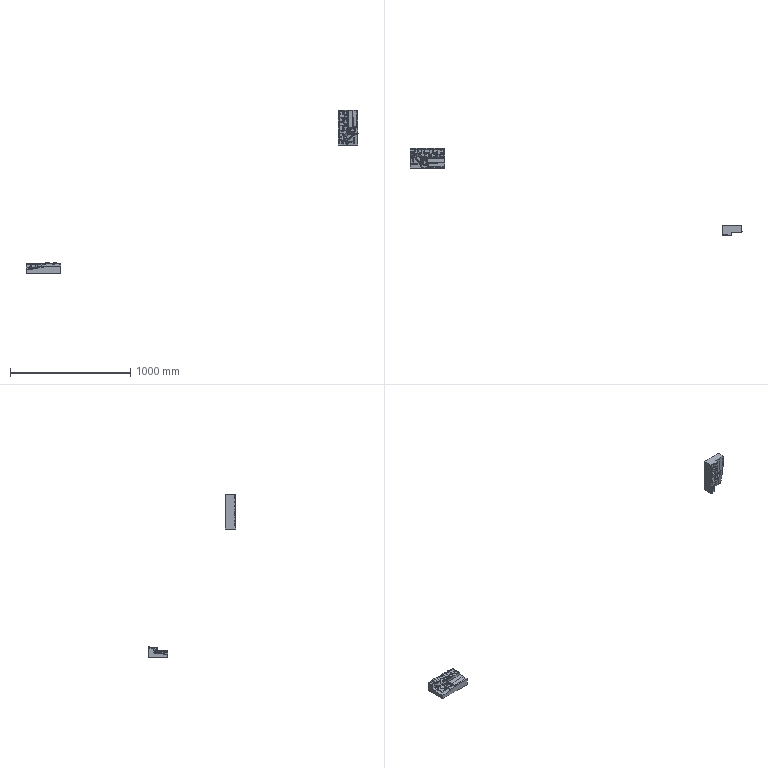Part | 2 solids | 820 faces | box 2756 x 729.572 x 1353 mm | volume 5861994 mm3 | spline 736 | plane 50 | cylinder 28 | sphere 6 | commonest cylinder face diameters 12.4 x16 7.6 x4 22.4 x4 13.6 x2 24.4 x2